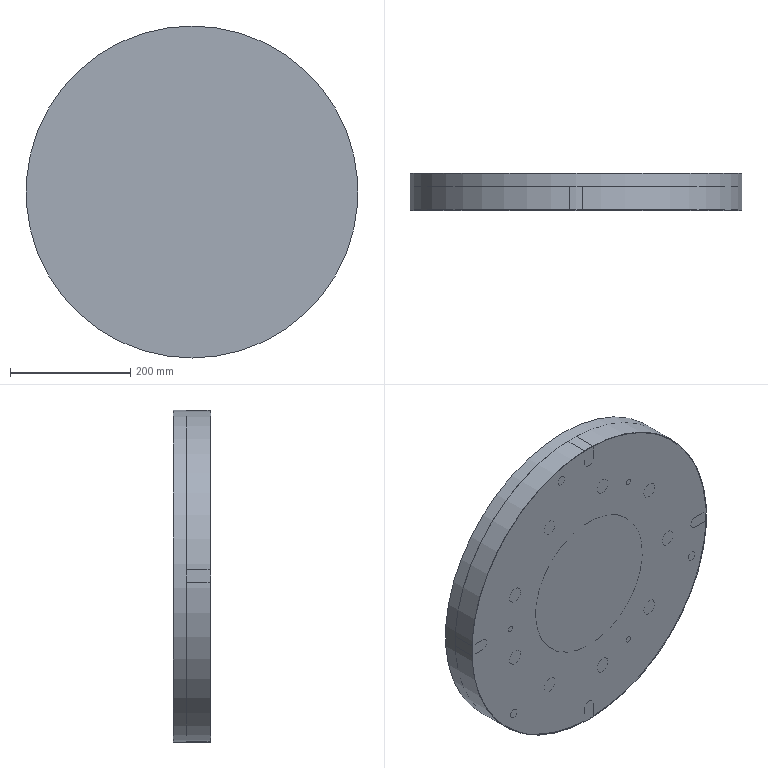NC program | NX | posted with a generic post | part box 552 x 62 x 552 mm
Whole program:
N10 G17 G21 G94 G90
(9-28槽_COPY , TOOL : D18)
N12 T02 M6
N14 G54
N16 G17 G0 G90 X43.377 Y-217.036 S900 M3
N18 G43 Z19. H2
N20 Z-1.
N22 G94 G1 Z-4. F60.
N24 X40.981 Y-203.451
N26 X40.596 Y-201.264
N28 G2 X40.439 Y-200.546 R9.
N30 G1 X38.872 Y-191.659
N32 X29.024 Y-193.395
N34 X30.591 Y-202.282
N36 G2 X30.689 Y-203.011 R9.
N38 G1 X31.075 Y-205.202
N40 X33.47 Y-218.783
N42 Z-1.
N44 G0 Z-0.8
N46 X43.377 Y-217.036
N48 Z-4.
N50 G1 Z-7.
N52 X40.981 Y-203.451
N54 X40.596 Y-201.264
N56 G2 X40.439 Y-200.546 R9.
N58 G1 X38.872 Y-191.659
N60 X29.024 Y-193.395
N62 X30.591 Y-202.282
N64 G2 X30.689 Y-203.011 R9.
N66 G1 X31.075 Y-205.202
N68 X33.47 Y-218.783
N70 Z-4.
N72 G0 Z19.
N74 M5
N76 M2